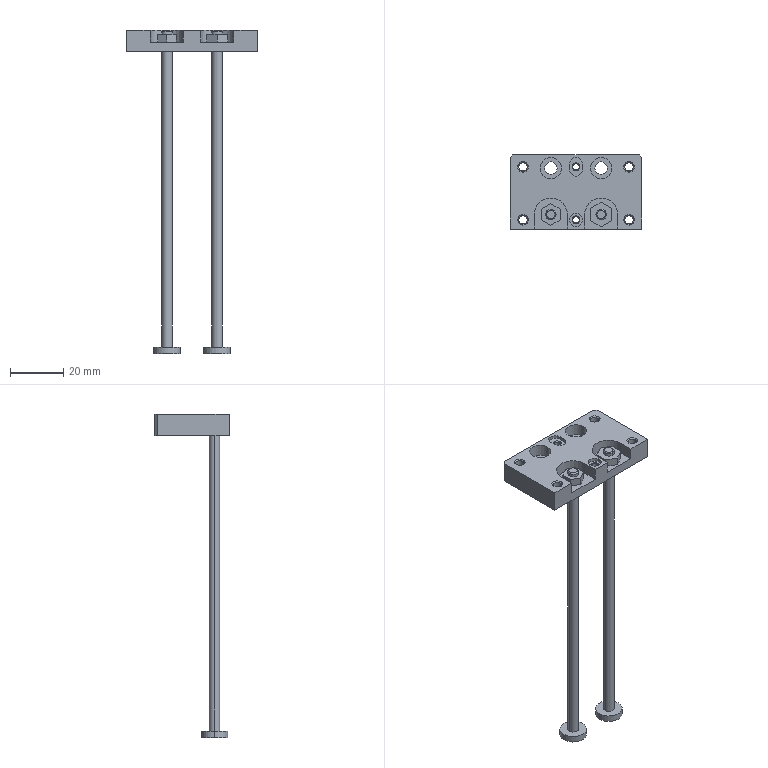Part | STEP file | 1 solid | 121 faces | box 49.6 x 28 x 122 mm | volume 12171 mm3 | plane 45 | cylinder 42 | cone 34 | commonest cylinder face diameters 3.2 x8 4 x8 2.4 x4 3 x4 4.7 x4 5 x4